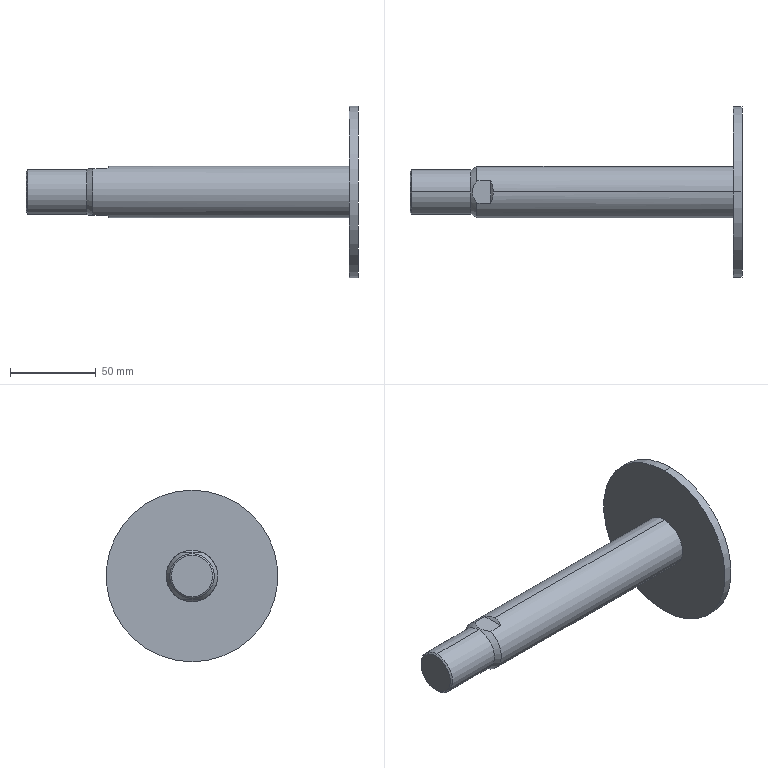Part | STEP file | 1 solid | 17 faces | box 193.5 x 100 x 100 mm | volume 165666 mm3 | plane 7 | cylinder 6 | cone 4 | commonest cylinder face diameters 26 x2 30 x2 100 x2